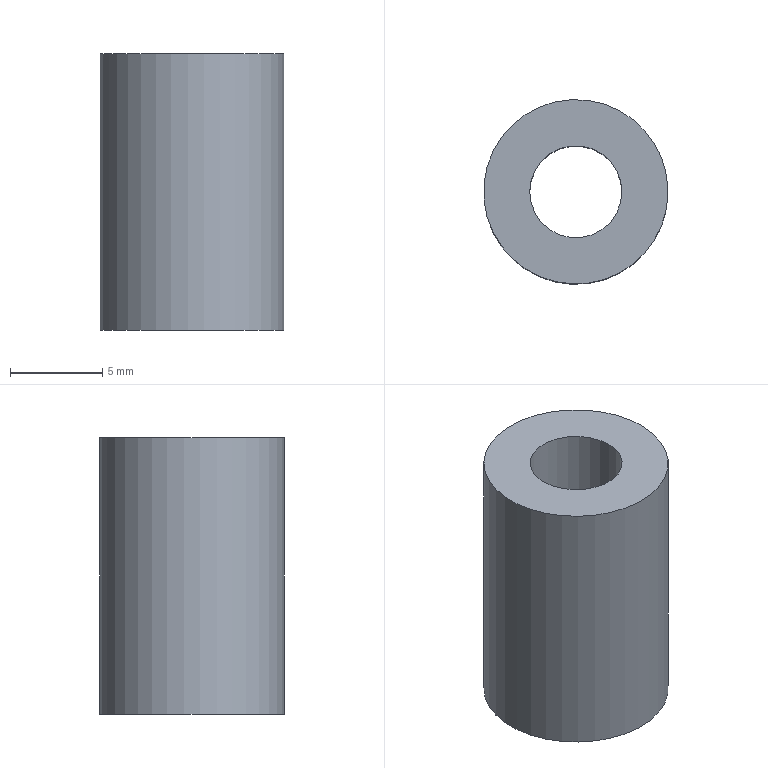Part | STEP file | gslz 2016.10.28-10_id1786_x_t | 1 solid | 4 faces | box 10 x 10 x 15 mm | volume 883.573 mm3 | cylinder 2 | plane 2 | commonest cylinder face diameters 5 x1 10 x1
STEP:
#1=CARTESIAN_POINT('',(0.,0.,0.));
#2=DIRECTION('',(0.,0.,1.));
#3=DIRECTION('',(1.,0.,0.));
#4=AXIS2_PLACEMENT_3D('',#1,#2,#3);
#5=CARTESIAN_POINT('',(914.5,119.5,25.));
#6=VERTEX_POINT('',#5);
#7=CARTESIAN_POINT('',(909.5,119.5,25.));
#8=DIRECTION('',(0.,0.,-1.));
#9=DIRECTION('',(1.,0.,0.));
#10=AXIS2_PLACEMENT_3D('',#7,#8,#9);
#11=CIRCLE('',#10,5.);
#12=CARTESIAN_POINT('',(909.5,119.5,35.));
#13=DIRECTION('',(0.,0.,-1.));
#14=DIRECTION('',(-1.,0.,0.));
#15=AXIS2_PLACEMENT_3D('',#12,#13,#14);
#16=CYLINDRICAL_SURFACE('',#15,5.);
#17=CARTESIAN_POINT('',(3.142,10.));
#18=DIRECTION('',(1.,0.));
#19=VECTOR('',#18,1.);
#20=LINE('',#17,#19);
#21=(GEOMETRIC_REPRESENTATION_CONTEXT(2)PARAMETRIC_REPRESENTATION_CONTEXT()REPRESENTATION_CONTEXT('',''));
#22=DEFINITIONAL_REPRESENTATION('',(#20),#21);
#23=PCURVE('',#16,#22);
#24=CARTESIAN_POINT('',(909.5,119.5,25.));
#25=DIRECTION('',(0.,0.,1.));
#26=DIRECTION('',(1.,0.,0.));
#27=AXIS2_PLACEMENT_3D('',#24,#25,#26);
#28=PLANE('',#27);
#29=CARTESIAN_POINT('',(5.,0.));
#30=CARTESIAN_POINT('',(5.,-8.66));
#31=CARTESIAN_POINT('',(-2.5,-4.33));
#32=CARTESIAN_POINT('',(-10.,0.));
#33=CARTESIAN_POINT('',(-2.5,4.33));
#34=CARTESIAN_POINT('',(5.,8.66));
#35=CARTESIAN_POINT('',(5.,0.));
#36=(BOUNDED_CURVE()B_SPLINE_CURVE(2,(#29,#30,#31,#32,#33,#34,#35),.UNSPECIFIED.,.T.,.F.)B_SPLINE_CURVE_WITH_KNOTS((1,2,2,2,2,1),(-2.094,0.,2.094,4.189,6.283,8.378),.UNSPECIFIED.)CURVE()GEOMETRIC_REPRESENTATION_ITEM()RATIONAL_B_SPLINE_CURVE((1.,0.5,1.,0.5,1.,0.5,1.))REPRESENTATION_ITEM(''));
#37=(GEOMETRIC_REPRESENTATION_CONTEXT(2)PARAMETRIC_REPRESENTATION_CONTEXT()REPRESENTATION_CONTEXT('',''));
#38=DEFINITIONAL_REPRESENTATION('',(#36),#37);
#39=PCURVE('',#28,#38);
#40=SURFACE_CURVE('',#11,(#23,#39),.PCURVE_S1.);
#41=EDGE_CURVE('',#6,#6,#40,.T.);
#42=ORIENTED_EDGE('',*,*,#41,.T.);
#43=CARTESIAN_POINT('',(914.5,119.5,10.));
#44=VERTEX_POINT('',#43);
#45=CARTESIAN_POINT('',(914.5,119.5,25.));
#46=CARTESIAN_POINT('',(914.5,119.5,10.));
#47=B_SPLINE_CURVE_WITH_KNOTS('',1,(#45,#46),.UNSPECIFIED.,.F.,.F.,(2,2),(10.,25.),.PIECEWISE_BEZIER_KNOTS.);
#48=CARTESIAN_POINT('',(9.425,0.));
#49=DIRECTION('',(0.,1.));
#50=VECTOR('',#49,1.);
#51=LINE('',#48,#50);
#52=(GEOMETRIC_REPRESENTATION_CONTEXT(2)PARAMETRIC_REPRESENTATION_CONTEXT()REPRESENTATION_CONTEXT('',''));
#53=DEFINITIONAL_REPRESENTATION('',(#51),#52);
#54=PCURVE('',#16,#53);
#55=CARTESIAN_POINT('',(3.142,0.));
#56=DIRECTION('',(0.,1.));
#57=VECTOR('',#56,1.);
#58=LINE('',#55,#57);
#59=(GEOMETRIC_REPRESENTATION_CONTEXT(2)PARAMETRIC_REPRESENTATION_CONTEXT()REPRESENTATION_CONTEXT('',''));
#60=DEFINITIONAL_REPRESENTATION('',(#58),#59);
#61=PCURVE('',#16,#60);
#62=SEAM_CURVE('',#47,(#54,#61),.PCURVE_S1.);
#63=EDGE_CURVE('',#6,#44,#62,.T.);
#64=ORIENTED_EDGE('',*,*,#63,.T.);
#65=CARTESIAN_POINT('',(909.5,119.5,10.));
#66=DIRECTION('',(0.,0.,-1.));
#67=DIRECTION('',(1.,0.,0.));
#68=AXIS2_PLACEMENT_3D('',#65,#66,#67);
#69=CIRCLE('',#68,5.);
#70=CARTESIAN_POINT('',(3.142,25.));
#71=DIRECTION('',(1.,0.));
#72=VECTOR('',#71,1.);
#73=LINE('',#70,#72);
#74=(GEOMETRIC_REPRESENTATION_CONTEXT(2)PARAMETRIC_REPRESENTATION_CONTEXT()REPRESENTATION_CONTEXT('',''));
#75=DEFINITIONAL_REPRESENTATION('',(#73),#74);
#76=PCURVE('',#16,#75);
#77=CARTESIAN_POINT('',(909.5,119.5,10.));
#78=DIRECTION('',(0.,0.,1.));
#79=DIRECTION('',(1.,0.,0.));
#80=AXIS2_PLACEMENT_3D('',#77,#78,#79);
#81=PLANE('',#80);
#82=CARTESIAN_POINT('',(5.,0.));
#83=CARTESIAN_POINT('',(5.,-8.66));
#84=CARTESIAN_POINT('',(-2.5,-4.33));
#85=CARTESIAN_POINT('',(-10.,0.));
#86=CARTESIAN_POINT('',(-2.5,4.33));
#87=CARTESIAN_POINT('',(5.,8.66));
#88=CARTESIAN_POINT('',(5.,0.));
#89=(BOUNDED_CURVE()B_SPLINE_CURVE(2,(#82,#83,#84,#85,#86,#87,#88),.UNSPECIFIED.,.T.,.F.)B_SPLINE_CURVE_WITH_KNOTS((1,2,2,2,2,1),(-2.094,0.,2.094,4.189,6.283,8.378),.UNSPECIFIED.)CURVE()GEOMETRIC_REPRESENTATION_ITEM()RATIONAL_B_SPLINE_CURVE((1.,0.5,1.,0.5,1.,0.5,1.))REPRESENTATION_ITEM(''));
#90=(GEOMETRIC_REPRESENTATION_CONTEXT(2)PARAMETRIC_REPRESENTATION_CONTEXT()REPRESENTATION_CONTEXT('',''));
#91=DEFINITIONAL_REPRESENTATION('',(#89),#90);
#92=PCURVE('',#81,#91);
#93=SURFACE_CURVE('',#69,(#76,#92),.PCURVE_S1.);
#94=EDGE_CURVE('',#44,#44,#93,.T.);
#95=ORIENTED_EDGE('',*,*,#94,.F.);
#96=ORIENTED_EDGE('',*,*,#63,.F.);
#97=EDGE_LOOP('',(#42,#64,#95,#96));
#98=FACE_BOUND('',#97,.T.);
#99=ADVANCED_FACE('',(#98),#16,.T.);
#100=CARTESIAN_POINT('',(912.,119.5,25.));
#101=VERTEX_POINT('',#100);
#102=CARTESIAN_POINT('',(909.5,119.5,25.));
#103=DIRECTION('',(0.,0.,-1.));
#104=DIRECTION('',(1.,0.,0.));
#105=AXIS2_PLACEMENT_3D('',#102,#103,#104);
#106=CIRCLE('',#105,2.5);
#107=CARTESIAN_POINT('',(909.5,119.5,35.));
#108=DIRECTION('',(0.,0.,-1.));
#109=DIRECTION('',(-1.,0.,0.));
#110=AXIS2_PLACEMENT_3D('',#107,#108,#109);
#111=CYLINDRICAL_SURFACE('',#110,2.5);
#112=CARTESIAN_POINT('',(3.142,10.));
#113=DIRECTION('',(1.,0.));
#114=VECTOR('',#113,1.);
#115=LINE('',#112,#114);
#116=(GEOMETRIC_REPRESENTATION_CONTEXT(2)PARAMETRIC_REPRESENTATION_CONTEXT()REPRESENTATION_CONTEXT('',''));
#117=DEFINITIONAL_REPRESENTATION('',(#115),#116);
#118=PCURVE('',#111,#117);
#119=CARTESIAN_POINT('',(2.5,0.));
#120=CARTESIAN_POINT('',(2.5,-4.33));
#121=CARTESIAN_POINT('',(-1.25,-2.165));
#122=CARTESIAN_POINT('',(-5.,0.));
#123=CARTESIAN_POINT('',(-1.25,2.165));
#124=CARTESIAN_POINT('',(2.5,4.33));
#125=CARTESIAN_POINT('',(2.5,0.));
#126=(BOUNDED_CURVE()B_SPLINE_CURVE(2,(#119,#120,#121,#122,#123,#124,#125),.UNSPECIFIED.,.T.,.F.)B_SPLINE_CURVE_WITH_KNOTS((1,2,2,2,2,1),(-2.094,0.,2.094,4.189,6.283,8.378),.UNSPECIFIED.)CURVE()GEOMETRIC_REPRESENTATION_ITEM()RATIONAL_B_SPLINE_CURVE((1.,0.5,1.,0.5,1.,0.5,1.))REPRESENTATION_ITEM(''));
#127=(GEOMETRIC_REPRESENTATION_CONTEXT(2)PARAMETRIC_REPRESENTATION_CONTEXT()REPRESENTATION_CONTEXT('',''));
#128=DEFINITIONAL_REPRESENTATION('',(#126),#127);
#129=PCURVE('',#28,#128);
#130=SURFACE_CURVE('',#106,(#118,#129),.PCURVE_S1.);
#131=EDGE_CURVE('',#101,#101,#130,.T.);
#132=ORIENTED_EDGE('',*,*,#131,.T.);
#133=CARTESIAN_POINT('',(912.,119.5,10.));
#134=VERTEX_POINT('',#133);
#135=CARTESIAN_POINT('',(912.,119.5,25.));
#136=CARTESIAN_POINT('',(912.,119.5,10.));
#137=B_SPLINE_CURVE_WITH_KNOTS('',1,(#135,#136),.UNSPECIFIED.,.F.,.F.,(2,2),(10.,25.),.PIECEWISE_BEZIER_KNOTS.);
#138=CARTESIAN_POINT('',(9.425,0.));
#139=DIRECTION('',(0.,1.));
#140=VECTOR('',#139,1.);
#141=LINE('',#138,#140);
#142=(GEOMETRIC_REPRESENTATION_CONTEXT(2)PARAMETRIC_REPRESENTATION_CONTEXT()REPRESENTATION_CONTEXT('',''));
#143=DEFINITIONAL_REPRESENTATION('',(#141),#142);
#144=PCURVE('',#111,#143);
#145=CARTESIAN_POINT('',(3.142,0.));
#146=DIRECTION('',(0.,1.));
#147=VECTOR('',#146,1.);
#148=LINE('',#145,#147);
#149=(GEOMETRIC_REPRESENTATION_CONTEXT(2)PARAMETRIC_REPRESENTATION_CONTEXT()REPRESENTATION_CONTEXT('',''));
#150=DEFINITIONAL_REPRESENTATION('',(#148),#149);
#151=PCURVE('',#111,#150);
#152=SEAM_CURVE('',#137,(#144,#151),.PCURVE_S1.);
#153=EDGE_CURVE('',#101,#134,#152,.T.);
#154=ORIENTED_EDGE('',*,*,#153,.T.);
#155=CARTESIAN_POINT('',(909.5,119.5,10.));
#156=DIRECTION('',(0.,0.,-1.));
#157=DIRECTION('',(1.,0.,0.));
#158=AXIS2_PLACEMENT_3D('',#155,#156,#157);
#159=CIRCLE('',#158,2.5);
#160=CARTESIAN_POINT('',(3.142,25.));
#161=DIRECTION('',(1.,0.));
#162=VECTOR('',#161,1.);
#163=LINE('',#160,#162);
#164=(GEOMETRIC_REPRESENTATION_CONTEXT(2)PARAMETRIC_REPRESENTATION_CONTEXT()REPRESENTATION_CONTEXT('',''));
#165=DEFINITIONAL_REPRESENTATION('',(#163),#164);
#166=PCURVE('',#111,#165);
#167=CARTESIAN_POINT('',(2.5,0.));
#168=CARTESIAN_POINT('',(2.5,-4.33));
#169=CARTESIAN_POINT('',(-1.25,-2.165));
#170=CARTESIAN_POINT('',(-5.,0.));
#171=CARTESIAN_POINT('',(-1.25,2.165));
#172=CARTESIAN_POINT('',(2.5,4.33));
#173=CARTESIAN_POINT('',(2.5,0.));
#174=(BOUNDED_CURVE()B_SPLINE_CURVE(2,(#167,#168,#169,#170,#171,#172,#173),.UNSPECIFIED.,.T.,.F.)B_SPLINE_CURVE_WITH_KNOTS((1,2,2,2,2,1),(-2.094,0.,2.094,4.189,6.283,8.378),.UNSPECIFIED.)CURVE()GEOMETRIC_REPRESENTATION_ITEM()RATIONAL_B_SPLINE_CURVE((1.,0.5,1.,0.5,1.,0.5,1.))REPRESENTATION_ITEM(''));
#175=(GEOMETRIC_REPRESENTATION_CONTEXT(2)PARAMETRIC_REPRESENTATION_CONTEXT()REPRESENTATION_CONTEXT('',''));
#176=DEFINITIONAL_REPRESENTATION('',(#174),#175);
#177=PCURVE('',#81,#176);
#178=SURFACE_CURVE('',#159,(#166,#177),.PCURVE_S1.);
#179=EDGE_CURVE('',#134,#134,#178,.T.);
#180=ORIENTED_EDGE('',*,*,#179,.F.);
#181=ORIENTED_EDGE('',*,*,#153,.F.);
#182=EDGE_LOOP('',(#132,#154,#180,#181));
#183=FACE_BOUND('',#182,.F.);
#184=ADVANCED_FACE('',(#183),#111,.F.);
#185=ORIENTED_EDGE('',*,*,#41,.F.);
#186=EDGE_LOOP('',(#185));
#187=FACE_BOUND('',#186,.T.);
#188=ORIENTED_EDGE('',*,*,#131,.T.);
#189=EDGE_LOOP('',(#188));
#190=FACE_BOUND('',#189,.T.);
#191=ADVANCED_FACE('',(#187,#190),#28,.T.);
#192=ORIENTED_EDGE('',*,*,#94,.T.);
#193=EDGE_LOOP('',(#192));
#194=FACE_BOUND('',#193,.T.);
#195=ORIENTED_EDGE('',*,*,#179,.F.);
#196=EDGE_LOOP('',(#195));
#197=FACE_BOUND('',#196,.T.);
#198=ADVANCED_FACE('',(#194,#197),#81,.F.);
#199=CLOSED_SHELL('',(#99,#184,#191,#198));
#200=MANIFOLD_SOLID_BREP('',#199);
#201=(LENGTH_UNIT()NAMED_UNIT(*)SI_UNIT(.MILLI.,.METRE.));
#202=UNCERTAINTY_MEASURE_WITH_UNIT(LENGTH_MEASURE(0.00001),#201,'','');
#203=(NAMED_UNIT(*)PLANE_ANGLE_UNIT()SI_UNIT($,.RADIAN.));
#204=(NAMED_UNIT(*)SI_UNIT($,.STERADIAN.)SOLID_ANGLE_UNIT());
#205=(GEOMETRIC_REPRESENTATION_CONTEXT(3)GLOBAL_UNCERTAINTY_ASSIGNED_CONTEXT((#202))GLOBAL_UNIT_ASSIGNED_CONTEXT((#201,#203,#204))REPRESENTATION_CONTEXT('',''));
#206=ADVANCED_BREP_SHAPE_REPRESENTATION('',(#4,#200),#205);